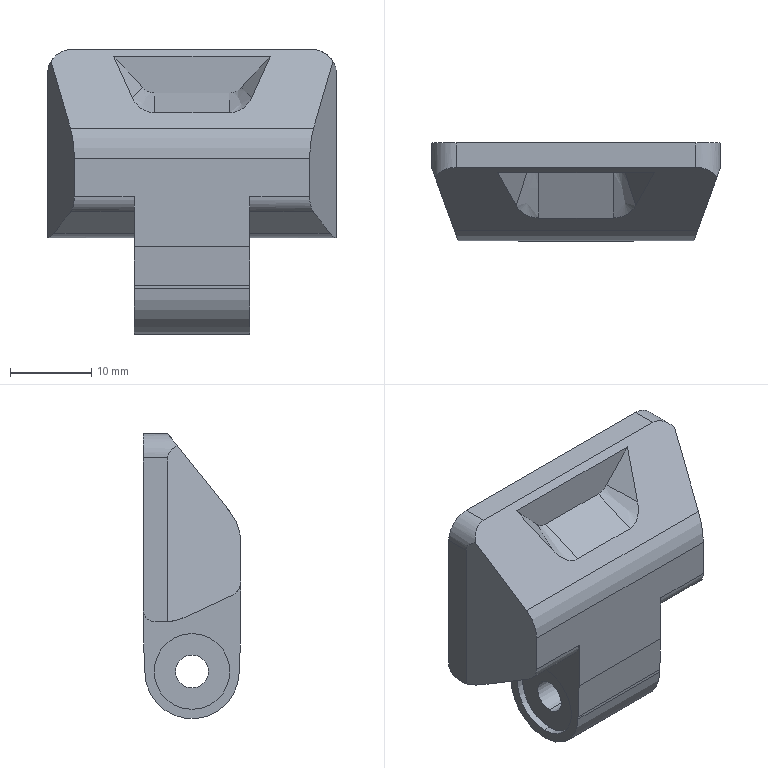Part | SolidWorks | features BaseBody 1 | 1 solid | 128 faces | box 35.464 x 12 x 35.016 mm | volume 8369 mm3 | cylinder 88 | plane 24 | cone 12 | spline 4 | commonest cylinder face diameters 5 x40 4.4 x31 9.3 x4 12 x3 3 x2 4 x2